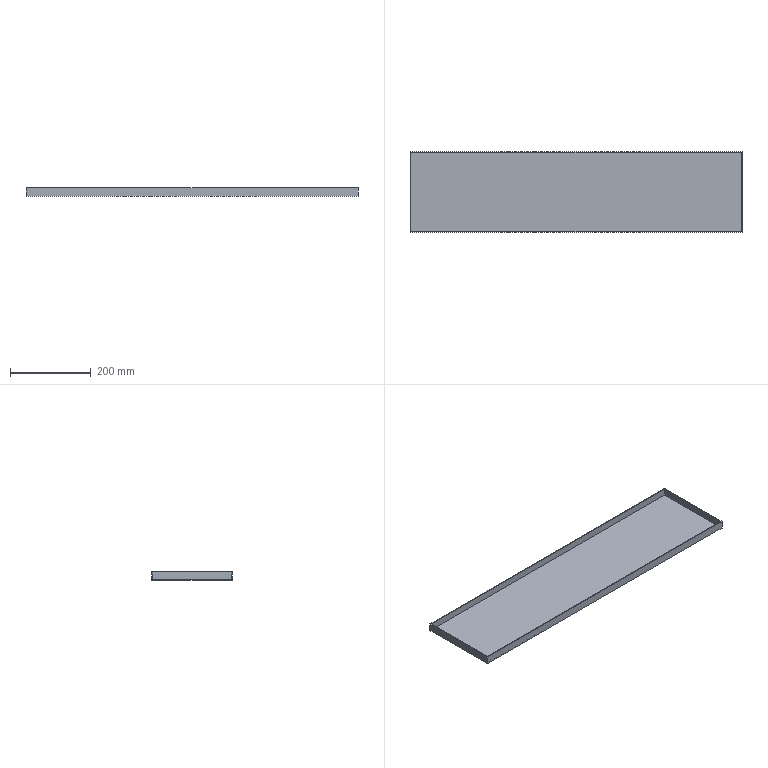Part | SolidWorks | features BaseBody 1 | 1 solid | 11 faces | box 820 x 200 x 20 mm | volume 401152 mm3 | plane 11
STEP:
#1=CARTESIAN_POINT('',(410.,-100.,-20.));
#2=VERTEX_POINT('',#1);
#3=CARTESIAN_POINT('',(410.,100.,-20.));
#4=VERTEX_POINT('',#3);
#5=CARTESIAN_POINT('',(410.,0.,-20.));
#6=DIRECTION('',(0.,1.,0.));
#7=VECTOR('',#6,1000.);
#8=LINE('',#5,#7);
#9=EDGE_CURVE('',#2,#4,#8,.T.);
#10=ORIENTED_EDGE('',*,*,#9,.T.);
#11=CARTESIAN_POINT('',(410.,100.,0.));
#12=VERTEX_POINT('',#11);
#13=CARTESIAN_POINT('',(410.,100.,-10.));
#14=DIRECTION('',(0.,0.,1.));
#15=VECTOR('',#14,1000.);
#16=LINE('',#13,#15);
#17=EDGE_CURVE('',#4,#12,#16,.T.);
#18=ORIENTED_EDGE('',*,*,#17,.T.);
#19=CARTESIAN_POINT('',(410.,-100.,0.));
#20=VERTEX_POINT('',#19);
#21=CARTESIAN_POINT('',(410.,0.,0.));
#22=DIRECTION('',(0.,-1.,0.));
#23=VECTOR('',#22,1000.);
#24=LINE('',#21,#23);
#25=EDGE_CURVE('',#12,#20,#24,.T.);
#26=ORIENTED_EDGE('',*,*,#25,.T.);
#27=CARTESIAN_POINT('',(410.,-100.,-10.));
#28=DIRECTION('',(0.,0.,-1.));
#29=VECTOR('',#28,1000.);
#30=LINE('',#27,#29);
#31=EDGE_CURVE('',#20,#2,#30,.T.);
#32=ORIENTED_EDGE('',*,*,#31,.T.);
#33=EDGE_LOOP('',(#10,#18,#26,#32));
#34=FACE_OUTER_BOUND('',#33,.T.);
#35=CARTESIAN_POINT('',(410.,-100.,0.));
#36=DIRECTION('',(1.,0.,0.));
#37=DIRECTION('',(0.,0.,-1.));
#38=AXIS2_PLACEMENT_3D('',#35,#36,#37);
#39=PLANE('',#38);
#40=ADVANCED_FACE('',(#34),#39,.T.);
#41=CARTESIAN_POINT('',(-410.,100.,-20.));
#42=VERTEX_POINT('',#41);
#43=CARTESIAN_POINT('',(0.,100.,-20.));
#44=DIRECTION('',(-1.,0.,0.));
#45=VECTOR('',#44,1000.);
#46=LINE('',#43,#45);
#47=EDGE_CURVE('',#4,#42,#46,.T.);
#48=ORIENTED_EDGE('',*,*,#47,.T.);
#49=CARTESIAN_POINT('',(-410.,100.,0.));
#50=VERTEX_POINT('',#49);
#51=CARTESIAN_POINT('',(-410.,100.,-10.));
#52=DIRECTION('',(0.,0.,1.));
#53=VECTOR('',#52,1000.);
#54=LINE('',#51,#53);
#55=EDGE_CURVE('',#42,#50,#54,.T.);
#56=ORIENTED_EDGE('',*,*,#55,.T.);
#57=CARTESIAN_POINT('',(0.,100.,0.));
#58=DIRECTION('',(1.,0.,0.));
#59=VECTOR('',#58,1000.);
#60=LINE('',#57,#59);
#61=EDGE_CURVE('',#50,#12,#60,.T.);
#62=ORIENTED_EDGE('',*,*,#61,.T.);
#63=ORIENTED_EDGE('',*,*,#17,.F.);
#64=EDGE_LOOP('',(#48,#56,#62,#63));
#65=FACE_OUTER_BOUND('',#64,.T.);
#66=CARTESIAN_POINT('',(-410.,100.,-20.));
#67=DIRECTION('',(0.,1.,0.));
#68=DIRECTION('',(0.,0.,1.));
#69=AXIS2_PLACEMENT_3D('',#66,#67,#68);
#70=PLANE('',#69);
#71=ADVANCED_FACE('',(#65),#70,.T.);
#72=CARTESIAN_POINT('',(-410.,-100.,-20.));
#73=VERTEX_POINT('',#72);
#74=CARTESIAN_POINT('',(-410.,0.,-20.));
#75=DIRECTION('',(0.,1.,0.));
#76=VECTOR('',#75,1000.);
#77=LINE('',#74,#76);
#78=EDGE_CURVE('',#73,#42,#77,.T.);
#79=ORIENTED_EDGE('',*,*,#78,.T.);
#80=ORIENTED_EDGE('',*,*,#47,.F.);
#81=ORIENTED_EDGE('',*,*,#9,.F.);
#82=CARTESIAN_POINT('',(0.,-100.,-20.));
#83=DIRECTION('',(-1.,0.,0.));
#84=VECTOR('',#83,1000.);
#85=LINE('',#82,#84);
#86=EDGE_CURVE('',#2,#73,#85,.T.);
#87=ORIENTED_EDGE('',*,*,#86,.T.);
#88=EDGE_LOOP('',(#79,#80,#81,#87));
#89=FACE_OUTER_BOUND('',#88,.T.);
#90=CARTESIAN_POINT('',(410.,-100.,-20.));
#91=DIRECTION('',(0.,0.,-1.));
#92=DIRECTION('',(-1.,0.,0.));
#93=AXIS2_PLACEMENT_3D('',#90,#91,#92);
#94=PLANE('',#93);
#95=ADVANCED_FACE('',(#89),#94,.T.);
#96=ORIENTED_EDGE('',*,*,#86,.F.);
#97=ORIENTED_EDGE('',*,*,#31,.F.);
#98=CARTESIAN_POINT('',(-410.,-100.,0.));
#99=VERTEX_POINT('',#98);
#100=CARTESIAN_POINT('',(0.,-100.,0.));
#101=DIRECTION('',(-1.,0.,0.));
#102=VECTOR('',#101,1000.);
#103=LINE('',#100,#102);
#104=EDGE_CURVE('',#20,#99,#103,.T.);
#105=ORIENTED_EDGE('',*,*,#104,.T.);
#106=CARTESIAN_POINT('',(-410.,-100.,-10.));
#107=DIRECTION('',(0.,0.,-1.));
#108=VECTOR('',#107,1000.);
#109=LINE('',#106,#108);
#110=EDGE_CURVE('',#99,#73,#109,.T.);
#111=ORIENTED_EDGE('',*,*,#110,.T.);
#112=EDGE_LOOP('',(#96,#97,#105,#111));
#113=FACE_OUTER_BOUND('',#112,.T.);
#114=CARTESIAN_POINT('',(-410.,-100.,0.));
#115=DIRECTION('',(0.,-1.,0.));
#116=DIRECTION('',(0.,0.,-1.));
#117=AXIS2_PLACEMENT_3D('',#114,#115,#116);
#118=PLANE('',#117);
#119=ADVANCED_FACE('',(#113),#118,.T.);
#120=CARTESIAN_POINT('',(-408.,98.,0.));
#121=VERTEX_POINT('',#120);
#122=CARTESIAN_POINT('',(-408.,-98.,0.));
#123=VERTEX_POINT('',#122);
#124=CARTESIAN_POINT('',(-408.,0.,0.));
#125=DIRECTION('',(0.,-1.,0.));
#126=VECTOR('',#125,1000.);
#127=LINE('',#124,#126);
#128=EDGE_CURVE('',#121,#123,#127,.T.);
#129=ORIENTED_EDGE('',*,*,#128,.F.);
#130=CARTESIAN_POINT('',(408.,98.,0.));
#131=VERTEX_POINT('',#130);
#132=CARTESIAN_POINT('',(0.,98.,0.));
#133=DIRECTION('',(-1.,0.,0.));
#134=VECTOR('',#133,1000.);
#135=LINE('',#132,#134);
#136=EDGE_CURVE('',#131,#121,#135,.T.);
#137=ORIENTED_EDGE('',*,*,#136,.F.);
#138=CARTESIAN_POINT('',(408.,-98.,0.));
#139=VERTEX_POINT('',#138);
#140=CARTESIAN_POINT('',(408.,0.,0.));
#141=DIRECTION('',(0.,1.,0.));
#142=VECTOR('',#141,1000.);
#143=LINE('',#140,#142);
#144=EDGE_CURVE('',#139,#131,#143,.T.);
#145=ORIENTED_EDGE('',*,*,#144,.F.);
#146=CARTESIAN_POINT('',(0.,-98.,0.));
#147=DIRECTION('',(1.,0.,0.));
#148=VECTOR('',#147,1000.);
#149=LINE('',#146,#148);
#150=EDGE_CURVE('',#123,#139,#149,.T.);
#151=ORIENTED_EDGE('',*,*,#150,.F.);
#152=EDGE_LOOP('',(#129,#137,#145,#151));
#153=FACE_BOUND('',#152,.T.);
#154=ORIENTED_EDGE('',*,*,#61,.F.);
#155=CARTESIAN_POINT('',(-410.,0.,0.));
#156=DIRECTION('',(0.,1.,0.));
#157=VECTOR('',#156,1000.);
#158=LINE('',#155,#157);
#159=EDGE_CURVE('',#99,#50,#158,.T.);
#160=ORIENTED_EDGE('',*,*,#159,.F.);
#161=ORIENTED_EDGE('',*,*,#104,.F.);
#162=ORIENTED_EDGE('',*,*,#25,.F.);
#163=EDGE_LOOP('',(#154,#160,#161,#162));
#164=FACE_OUTER_BOUND('',#163,.T.);
#165=CARTESIAN_POINT('',(410.,-100.,0.));
#166=DIRECTION('',(0.,0.,-1.));
#167=DIRECTION('',(-1.,0.,0.));
#168=AXIS2_PLACEMENT_3D('',#165,#166,#167);
#169=PLANE('',#168);
#170=ADVANCED_FACE('',(#153,#164),#169,.F.);
#171=ORIENTED_EDGE('',*,*,#78,.F.);
#172=ORIENTED_EDGE('',*,*,#110,.F.);
#173=ORIENTED_EDGE('',*,*,#159,.T.);
#174=ORIENTED_EDGE('',*,*,#55,.F.);
#175=EDGE_LOOP('',(#171,#172,#173,#174));
#176=FACE_OUTER_BOUND('',#175,.T.);
#177=CARTESIAN_POINT('',(-410.,-100.,-20.));
#178=DIRECTION('',(-1.,0.,0.));
#179=DIRECTION('',(0.,0.,1.));
#180=AXIS2_PLACEMENT_3D('',#177,#178,#179);
#181=PLANE('',#180);
#182=ADVANCED_FACE('',(#176),#181,.T.);
#183=CARTESIAN_POINT('',(408.,-98.,-18.));
#184=VERTEX_POINT('',#183);
#185=CARTESIAN_POINT('',(408.,-98.,-9.));
#186=DIRECTION('',(0.,0.,1.));
#187=VECTOR('',#186,1000.);
#188=LINE('',#185,#187);
#189=EDGE_CURVE('',#184,#139,#188,.T.);
#190=ORIENTED_EDGE('',*,*,#189,.F.);
#191=CARTESIAN_POINT('',(-408.,-98.,-18.));
#192=VERTEX_POINT('',#191);
#193=CARTESIAN_POINT('',(0.,-98.,-18.));
#194=DIRECTION('',(1.,0.,0.));
#195=VECTOR('',#194,1000.);
#196=LINE('',#193,#195);
#197=EDGE_CURVE('',#192,#184,#196,.T.);
#198=ORIENTED_EDGE('',*,*,#197,.F.);
#199=CARTESIAN_POINT('',(-408.,-98.,-9.));
#200=DIRECTION('',(0.,0.,-1.));
#201=VECTOR('',#200,1000.);
#202=LINE('',#199,#201);
#203=EDGE_CURVE('',#123,#192,#202,.T.);
#204=ORIENTED_EDGE('',*,*,#203,.F.);
#205=ORIENTED_EDGE('',*,*,#150,.T.);
#206=EDGE_LOOP('',(#190,#198,#204,#205));
#207=FACE_OUTER_BOUND('',#206,.T.);
#208=CARTESIAN_POINT('',(-408.,-98.,-18.));
#209=DIRECTION('',(0.,-1.,0.));
#210=DIRECTION('',(1.,0.,0.));
#211=AXIS2_PLACEMENT_3D('',#208,#209,#210);
#212=PLANE('',#211);
#213=ADVANCED_FACE('',(#207),#212,.F.);
#214=ORIENTED_EDGE('',*,*,#203,.T.);
#215=CARTESIAN_POINT('',(-408.,98.,-18.));
#216=VERTEX_POINT('',#215);
#217=CARTESIAN_POINT('',(-408.,0.,-18.));
#218=DIRECTION('',(0.,-1.,0.));
#219=VECTOR('',#218,1000.);
#220=LINE('',#217,#219);
#221=EDGE_CURVE('',#216,#192,#220,.T.);
#222=ORIENTED_EDGE('',*,*,#221,.F.);
#223=CARTESIAN_POINT('',(-408.,98.,-9.));
#224=DIRECTION('',(0.,0.,-1.));
#225=VECTOR('',#224,1000.);
#226=LINE('',#223,#225);
#227=EDGE_CURVE('',#121,#216,#226,.T.);
#228=ORIENTED_EDGE('',*,*,#227,.F.);
#229=ORIENTED_EDGE('',*,*,#128,.T.);
#230=EDGE_LOOP('',(#214,#222,#228,#229));
#231=FACE_OUTER_BOUND('',#230,.T.);
#232=CARTESIAN_POINT('',(-408.,-98.,-18.));
#233=DIRECTION('',(-1.,0.,0.));
#234=DIRECTION('',(0.,0.,1.));
#235=AXIS2_PLACEMENT_3D('',#232,#233,#234);
#236=PLANE('',#235);
#237=ADVANCED_FACE('',(#231),#236,.F.);
#238=ORIENTED_EDGE('',*,*,#227,.T.);
#239=CARTESIAN_POINT('',(408.,98.,-18.));
#240=VERTEX_POINT('',#239);
#241=CARTESIAN_POINT('',(0.,98.,-18.));
#242=DIRECTION('',(-1.,0.,0.));
#243=VECTOR('',#242,1000.);
#244=LINE('',#241,#243);
#245=EDGE_CURVE('',#240,#216,#244,.T.);
#246=ORIENTED_EDGE('',*,*,#245,.F.);
#247=CARTESIAN_POINT('',(408.,98.,-9.));
#248=DIRECTION('',(0.,0.,-1.));
#249=VECTOR('',#248,1000.);
#250=LINE('',#247,#249);
#251=EDGE_CURVE('',#131,#240,#250,.T.);
#252=ORIENTED_EDGE('',*,*,#251,.F.);
#253=ORIENTED_EDGE('',*,*,#136,.T.);
#254=EDGE_LOOP('',(#238,#246,#252,#253));
#255=FACE_OUTER_BOUND('',#254,.T.);
#256=CARTESIAN_POINT('',(408.,98.,-18.));
#257=DIRECTION('',(0.,1.,0.));
#258=DIRECTION('',(-1.,0.,0.));
#259=AXIS2_PLACEMENT_3D('',#256,#257,#258);
#260=PLANE('',#259);
#261=ADVANCED_FACE('',(#255),#260,.F.);
#262=ORIENTED_EDGE('',*,*,#251,.T.);
#263=CARTESIAN_POINT('',(408.,0.,-18.));
#264=DIRECTION('',(0.,1.,0.));
#265=VECTOR('',#264,1000.);
#266=LINE('',#263,#265);
#267=EDGE_CURVE('',#184,#240,#266,.T.);
#268=ORIENTED_EDGE('',*,*,#267,.F.);
#269=ORIENTED_EDGE('',*,*,#189,.T.);
#270=ORIENTED_EDGE('',*,*,#144,.T.);
#271=EDGE_LOOP('',(#262,#268,#269,#270));
#272=FACE_OUTER_BOUND('',#271,.T.);
#273=CARTESIAN_POINT('',(408.,-98.,0.));
#274=DIRECTION('',(1.,0.,0.));
#275=DIRECTION('',(0.,0.,-1.));
#276=AXIS2_PLACEMENT_3D('',#273,#274,#275);
#277=PLANE('',#276);
#278=ADVANCED_FACE('',(#272),#277,.F.);
#279=ORIENTED_EDGE('',*,*,#267,.T.);
#280=ORIENTED_EDGE('',*,*,#245,.T.);
#281=ORIENTED_EDGE('',*,*,#221,.T.);
#282=ORIENTED_EDGE('',*,*,#197,.T.);
#283=EDGE_LOOP('',(#279,#280,#281,#282));
#284=FACE_OUTER_BOUND('',#283,.T.);
#285=CARTESIAN_POINT('',(-408.,-98.,-18.));
#286=DIRECTION('',(0.,0.,1.));
#287=DIRECTION('',(1.,0.,0.));
#288=AXIS2_PLACEMENT_3D('',#285,#286,#287);
#289=PLANE('',#288);
#290=ADVANCED_FACE('',(#284),#289,.T.);
#291=CLOSED_SHELL('',(#40,#71,#95,#119,#170,#182,#213,#237,#261,#278,#290));
#292=MANIFOLD_SOLID_BREP('',#291);
#293=CARTESIAN_POINT('',(0.,0.,0.));
#294=DIRECTION('',(0.,0.,1.));
#295=DIRECTION('',(1.,0.,0.));
#296=AXIS2_PLACEMENT_3D('',#293,#294,#295);
#297=(LENGTH_UNIT()NAMED_UNIT(*)SI_UNIT(.MILLI.,.METRE.));
#298=UNCERTAINTY_MEASURE_WITH_UNIT(LENGTH_MEASURE(0.00001),#297,'','');
#299=(NAMED_UNIT(*)PLANE_ANGLE_UNIT()SI_UNIT($,.RADIAN.));
#300=(NAMED_UNIT(*)SI_UNIT($,.STERADIAN.)SOLID_ANGLE_UNIT());
#301=(GEOMETRIC_REPRESENTATION_CONTEXT(3)GLOBAL_UNCERTAINTY_ASSIGNED_CONTEXT((#298))GLOBAL_UNIT_ASSIGNED_CONTEXT((#297,#299,#300))REPRESENTATION_CONTEXT('',''));
#302=ADVANCED_BREP_SHAPE_REPRESENTATION('',(#292,#296),#301);